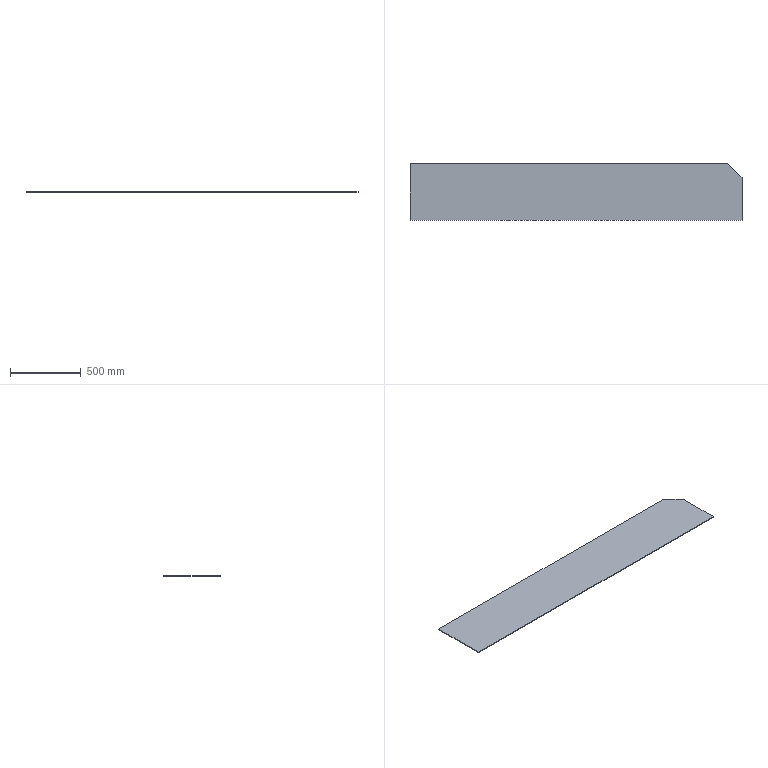Part | SolidWorks | features FlatPattern 1, SMBaseFlange 1, SheetMetal 1 | 1 solid | 7 faces | box 2350 x 400 x 5 mm | volume 4675000 mm3 | plane 7
STEP:
#1=CARTESIAN_POINT('',(0.,400.,0.));
#2=VERTEX_POINT('',#1);
#3=CARTESIAN_POINT('',(0.,0.,0.));
#4=VERTEX_POINT('',#3);
#5=CARTESIAN_POINT('',(0.,0.,0.));
#6=DIRECTION('',(0.,-1.,0.));
#7=VECTOR('',#6,1000.);
#8=LINE('',#5,#7);
#9=EDGE_CURVE('',#2,#4,#8,.T.);
#10=ORIENTED_EDGE('',*,*,#9,.F.);
#11=CARTESIAN_POINT('',(0.,400.,-5.));
#12=VERTEX_POINT('',#11);
#13=CARTESIAN_POINT('',(0.,400.,-5.));
#14=DIRECTION('',(0.,0.,1.));
#15=VECTOR('',#14,1000.);
#16=LINE('',#13,#15);
#17=EDGE_CURVE('',#12,#2,#16,.T.);
#18=ORIENTED_EDGE('',*,*,#17,.F.);
#19=CARTESIAN_POINT('',(0.,0.,-5.));
#20=VERTEX_POINT('',#19);
#21=CARTESIAN_POINT('',(0.,0.,-5.));
#22=DIRECTION('',(0.,-1.,0.));
#23=VECTOR('',#22,1000.);
#24=LINE('',#21,#23);
#25=EDGE_CURVE('',#12,#20,#24,.T.);
#26=ORIENTED_EDGE('',*,*,#25,.T.);
#27=CARTESIAN_POINT('',(0.,0.,-5.));
#28=DIRECTION('',(0.,0.,1.));
#29=VECTOR('',#28,1000.);
#30=LINE('',#27,#29);
#31=EDGE_CURVE('',#20,#4,#30,.T.);
#32=ORIENTED_EDGE('',*,*,#31,.T.);
#33=EDGE_LOOP('',(#10,#18,#26,#32));
#34=FACE_OUTER_BOUND('',#33,.T.);
#35=CARTESIAN_POINT('',(0.,0.,-5.));
#36=DIRECTION('',(-1.,0.,0.));
#37=DIRECTION('',(0.,0.,1.));
#38=AXIS2_PLACEMENT_3D('',#35,#36,#37);
#39=PLANE('',#38);
#40=ADVANCED_FACE('',(#34),#39,.T.);
#41=CARTESIAN_POINT('',(2250.,400.,0.));
#42=VERTEX_POINT('',#41);
#43=CARTESIAN_POINT('',(0.,400.,0.));
#44=DIRECTION('',(-1.,0.,0.));
#45=VECTOR('',#44,1000.);
#46=LINE('',#43,#45);
#47=EDGE_CURVE('',#42,#2,#46,.T.);
#48=ORIENTED_EDGE('',*,*,#47,.F.);
#49=CARTESIAN_POINT('',(2250.,400.,-5.));
#50=VERTEX_POINT('',#49);
#51=CARTESIAN_POINT('',(2250.,400.,-5.));
#52=DIRECTION('',(0.,0.,1.));
#53=VECTOR('',#52,1000.);
#54=LINE('',#51,#53);
#55=EDGE_CURVE('',#50,#42,#54,.T.);
#56=ORIENTED_EDGE('',*,*,#55,.F.);
#57=CARTESIAN_POINT('',(0.,400.,-5.));
#58=DIRECTION('',(-1.,0.,0.));
#59=VECTOR('',#58,1000.);
#60=LINE('',#57,#59);
#61=EDGE_CURVE('',#50,#12,#60,.T.);
#62=ORIENTED_EDGE('',*,*,#61,.T.);
#63=ORIENTED_EDGE('',*,*,#17,.T.);
#64=EDGE_LOOP('',(#48,#56,#62,#63));
#65=FACE_OUTER_BOUND('',#64,.T.);
#66=CARTESIAN_POINT('',(0.,400.,-5.));
#67=DIRECTION('',(0.,1.,0.));
#68=DIRECTION('',(0.,0.,1.));
#69=AXIS2_PLACEMENT_3D('',#66,#67,#68);
#70=PLANE('',#69);
#71=ADVANCED_FACE('',(#65),#70,.T.);
#72=CARTESIAN_POINT('',(2350.,300.,0.));
#73=VERTEX_POINT('',#72);
#74=CARTESIAN_POINT('',(2250.,400.,0.));
#75=DIRECTION('',(-0.7071,0.7071,0.));
#76=VECTOR('',#75,1000.);
#77=LINE('',#74,#76);
#78=EDGE_CURVE('',#73,#42,#77,.T.);
#79=ORIENTED_EDGE('',*,*,#78,.F.);
#80=CARTESIAN_POINT('',(2350.,300.,-5.));
#81=VERTEX_POINT('',#80);
#82=CARTESIAN_POINT('',(2350.,300.,-5.));
#83=DIRECTION('',(0.,0.,1.));
#84=VECTOR('',#83,1000.);
#85=LINE('',#82,#84);
#86=EDGE_CURVE('',#81,#73,#85,.T.);
#87=ORIENTED_EDGE('',*,*,#86,.F.);
#88=CARTESIAN_POINT('',(2250.,400.,-5.));
#89=DIRECTION('',(-0.7071,0.7071,0.));
#90=VECTOR('',#89,1000.);
#91=LINE('',#88,#90);
#92=EDGE_CURVE('',#81,#50,#91,.T.);
#93=ORIENTED_EDGE('',*,*,#92,.T.);
#94=ORIENTED_EDGE('',*,*,#55,.T.);
#95=EDGE_LOOP('',(#79,#87,#93,#94));
#96=FACE_OUTER_BOUND('',#95,.T.);
#97=CARTESIAN_POINT('',(2250.,400.,-5.));
#98=DIRECTION('',(0.7071,0.7071,0.));
#99=DIRECTION('',(-0.7071,0.7071,0.));
#100=AXIS2_PLACEMENT_3D('',#97,#98,#99);
#101=PLANE('',#100);
#102=ADVANCED_FACE('',(#96),#101,.T.);
#103=CARTESIAN_POINT('',(2350.,0.,0.));
#104=VERTEX_POINT('',#103);
#105=CARTESIAN_POINT('',(2350.,0.,0.));
#106=DIRECTION('',(0.,1.,0.));
#107=VECTOR('',#106,1000.);
#108=LINE('',#105,#107);
#109=EDGE_CURVE('',#104,#73,#108,.T.);
#110=ORIENTED_EDGE('',*,*,#109,.F.);
#111=CARTESIAN_POINT('',(2350.,0.,-5.));
#112=VERTEX_POINT('',#111);
#113=CARTESIAN_POINT('',(2350.,0.,-5.));
#114=DIRECTION('',(0.,0.,1.));
#115=VECTOR('',#114,1000.);
#116=LINE('',#113,#115);
#117=EDGE_CURVE('',#112,#104,#116,.T.);
#118=ORIENTED_EDGE('',*,*,#117,.F.);
#119=CARTESIAN_POINT('',(2350.,0.,-5.));
#120=DIRECTION('',(0.,1.,0.));
#121=VECTOR('',#120,1000.);
#122=LINE('',#119,#121);
#123=EDGE_CURVE('',#112,#81,#122,.T.);
#124=ORIENTED_EDGE('',*,*,#123,.T.);
#125=ORIENTED_EDGE('',*,*,#86,.T.);
#126=EDGE_LOOP('',(#110,#118,#124,#125));
#127=FACE_OUTER_BOUND('',#126,.T.);
#128=CARTESIAN_POINT('',(2350.,0.,-5.));
#129=DIRECTION('',(1.,0.,0.));
#130=DIRECTION('',(0.,0.,-1.));
#131=AXIS2_PLACEMENT_3D('',#128,#129,#130);
#132=PLANE('',#131);
#133=ADVANCED_FACE('',(#127),#132,.T.);
#134=CARTESIAN_POINT('',(0.,0.,0.));
#135=DIRECTION('',(1.,0.,0.));
#136=VECTOR('',#135,1000.);
#137=LINE('',#134,#136);
#138=EDGE_CURVE('',#4,#104,#137,.T.);
#139=ORIENTED_EDGE('',*,*,#138,.F.);
#140=ORIENTED_EDGE('',*,*,#31,.F.);
#141=CARTESIAN_POINT('',(0.,0.,-5.));
#142=DIRECTION('',(1.,0.,0.));
#143=VECTOR('',#142,1000.);
#144=LINE('',#141,#143);
#145=EDGE_CURVE('',#20,#112,#144,.T.);
#146=ORIENTED_EDGE('',*,*,#145,.T.);
#147=ORIENTED_EDGE('',*,*,#117,.T.);
#148=EDGE_LOOP('',(#139,#140,#146,#147));
#149=FACE_OUTER_BOUND('',#148,.T.);
#150=CARTESIAN_POINT('',(0.,0.,-5.));
#151=DIRECTION('',(0.,-1.,0.));
#152=DIRECTION('',(0.,0.,-1.));
#153=AXIS2_PLACEMENT_3D('',#150,#151,#152);
#154=PLANE('',#153);
#155=ADVANCED_FACE('',(#149),#154,.T.);
#156=ORIENTED_EDGE('',*,*,#25,.F.);
#157=ORIENTED_EDGE('',*,*,#61,.F.);
#158=ORIENTED_EDGE('',*,*,#92,.F.);
#159=ORIENTED_EDGE('',*,*,#123,.F.);
#160=ORIENTED_EDGE('',*,*,#145,.F.);
#161=EDGE_LOOP('',(#156,#157,#158,#159,#160));
#162=FACE_OUTER_BOUND('',#161,.T.);
#163=CARTESIAN_POINT('',(0.,0.,-5.));
#164=DIRECTION('',(0.,0.,-1.));
#165=DIRECTION('',(-1.,0.,0.));
#166=AXIS2_PLACEMENT_3D('',#163,#164,#165);
#167=PLANE('',#166);
#168=ADVANCED_FACE('',(#162),#167,.T.);
#169=ORIENTED_EDGE('',*,*,#9,.T.);
#170=ORIENTED_EDGE('',*,*,#138,.T.);
#171=ORIENTED_EDGE('',*,*,#109,.T.);
#172=ORIENTED_EDGE('',*,*,#78,.T.);
#173=ORIENTED_EDGE('',*,*,#47,.T.);
#174=EDGE_LOOP('',(#169,#170,#171,#172,#173));
#175=FACE_OUTER_BOUND('',#174,.T.);
#176=CARTESIAN_POINT('',(0.,0.,0.));
#177=DIRECTION('',(0.,0.,-1.));
#178=DIRECTION('',(-1.,0.,0.));
#179=AXIS2_PLACEMENT_3D('',#176,#177,#178);
#180=PLANE('',#179);
#181=ADVANCED_FACE('',(#175),#180,.F.);
#182=CLOSED_SHELL('',(#40,#71,#102,#133,#155,#168,#181));
#183=MANIFOLD_SOLID_BREP('',#182);
#184=CARTESIAN_POINT('',(0.,0.,0.));
#185=DIRECTION('',(0.,0.,1.));
#186=DIRECTION('',(1.,0.,0.));
#187=AXIS2_PLACEMENT_3D('',#184,#185,#186);
#188=(LENGTH_UNIT()NAMED_UNIT(*)SI_UNIT(.MILLI.,.METRE.));
#189=UNCERTAINTY_MEASURE_WITH_UNIT(LENGTH_MEASURE(0.00001),#188,'','');
#190=(NAMED_UNIT(*)PLANE_ANGLE_UNIT()SI_UNIT($,.RADIAN.));
#191=(NAMED_UNIT(*)SI_UNIT($,.STERADIAN.)SOLID_ANGLE_UNIT());
#192=(GEOMETRIC_REPRESENTATION_CONTEXT(3)GLOBAL_UNCERTAINTY_ASSIGNED_CONTEXT((#189))GLOBAL_UNIT_ASSIGNED_CONTEXT((#188,#190,#191))REPRESENTATION_CONTEXT('',''));
#193=ADVANCED_BREP_SHAPE_REPRESENTATION('',(#183,#187),#192);